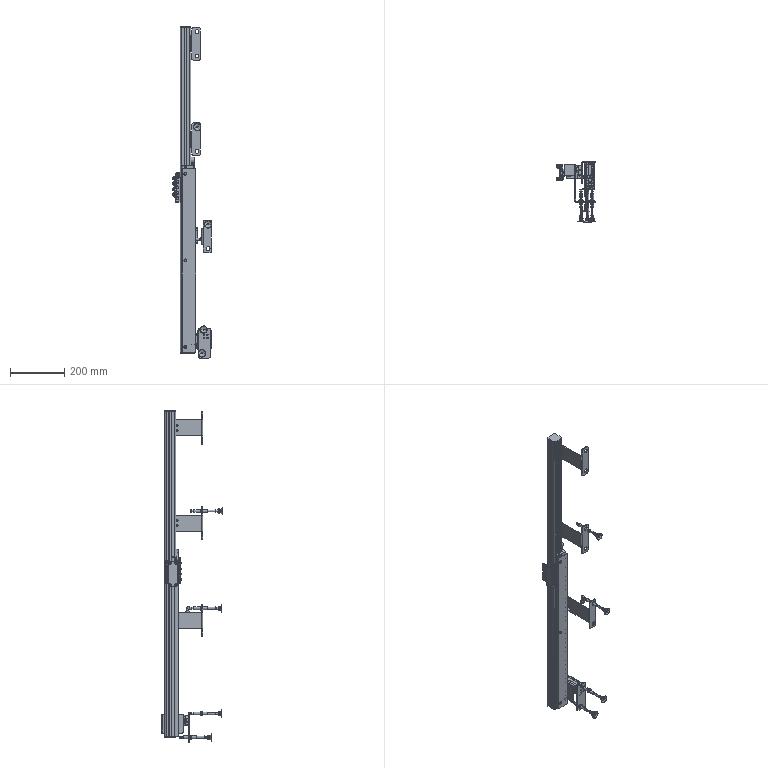Part | SolidWorks | features ReferencePattern 2, LocalLPattern 1, MirrorCompFeat 1 | 42 solids | 3315 faces | volume 1567936 mm3 | plane 1344 | cylinder 1057 | cone 650 | spline 264 | commonest cylinder face diameters 4.1 x66 4 x58 7 x57 10 x52 6 x50 4.2 x48